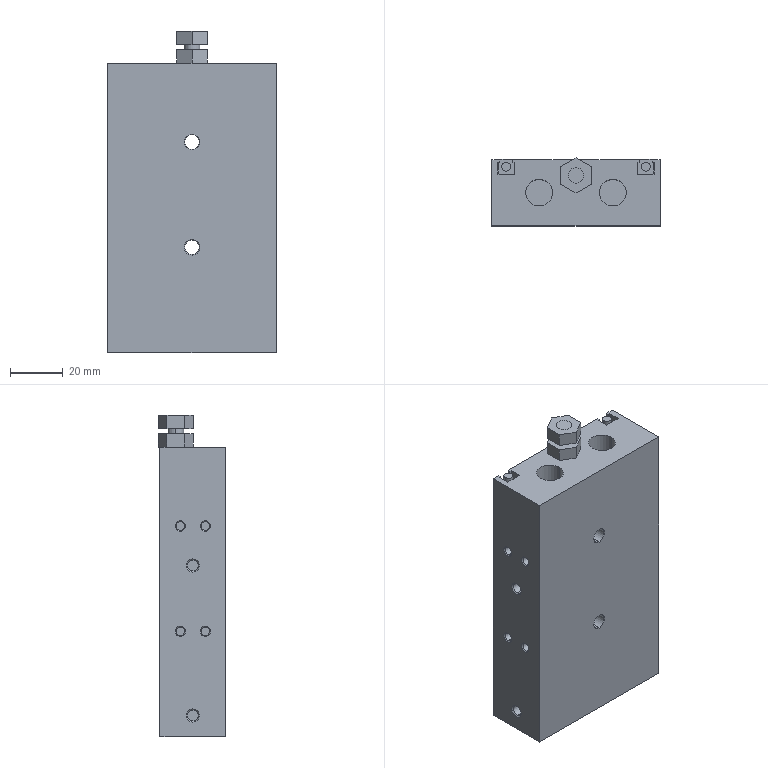Part | STEP file | body_A_CXSM20_40_Z80_0_ | 1 solid | 147 faces | box 64 x 25.64 x 122 mm | volume 162743 mm3 | plane 75 | cylinder 44 | cone 28 | commonest cylinder face diameters 3.24 x16 4.13 x8 3.4 x4 5.5 x4 6 x4 9.5 x4